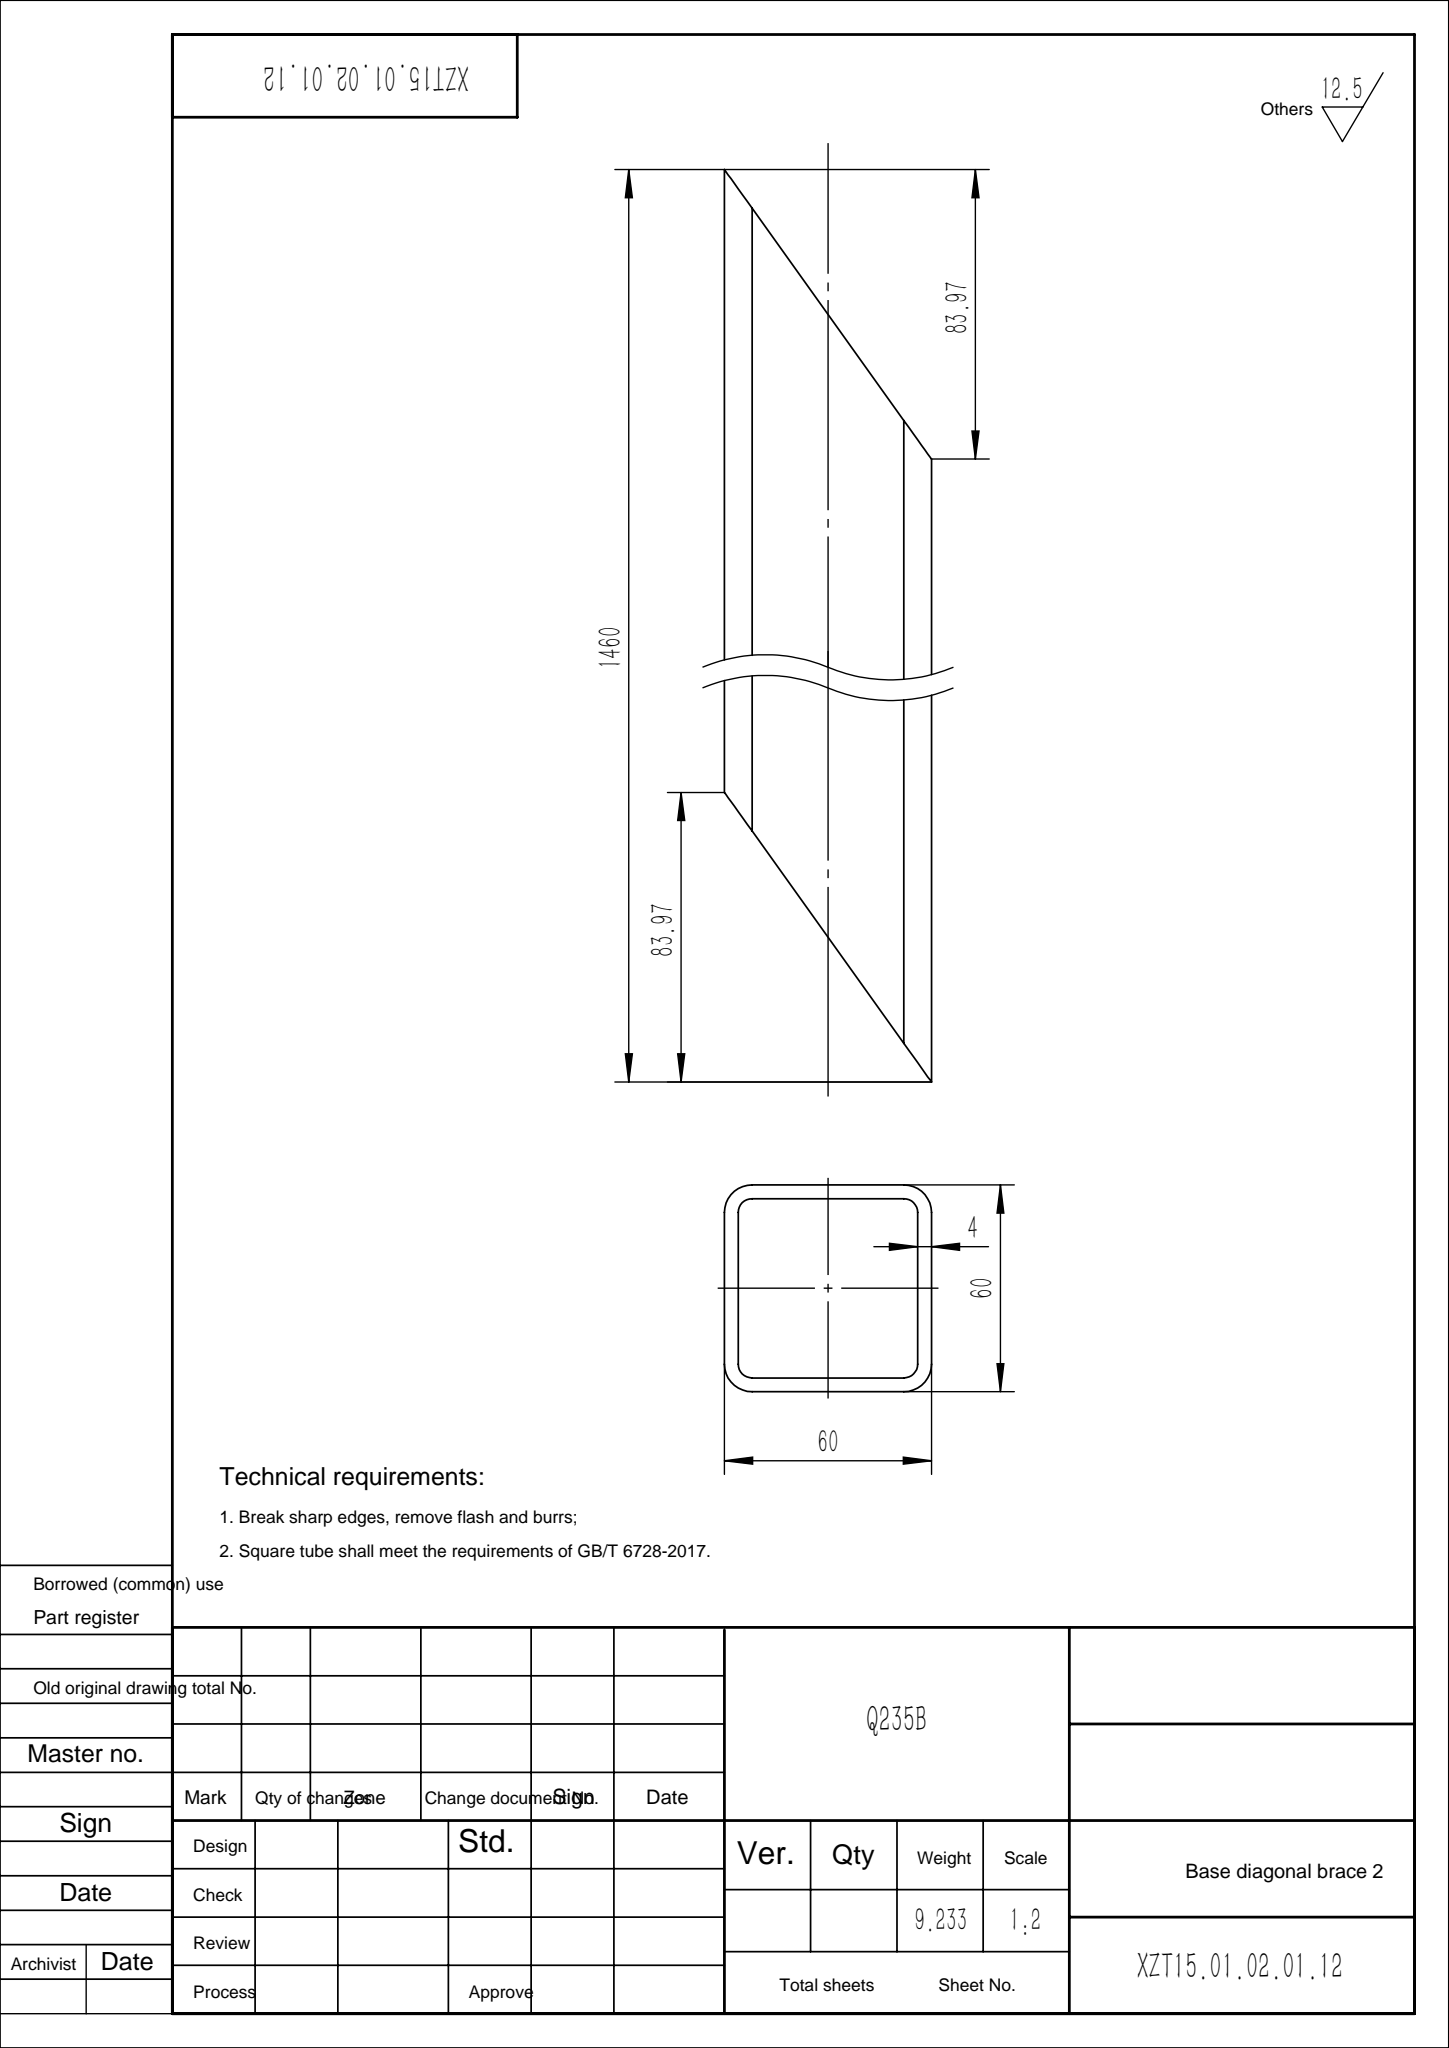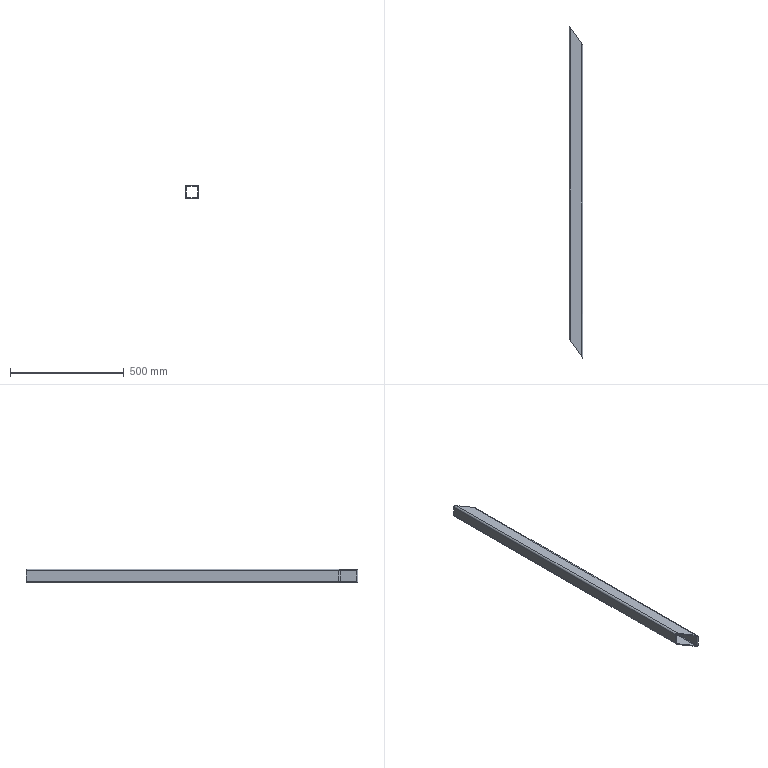Part | SolidWorks | features ICE 1, WeldMemberFeat 1, WeldmentFeature 1 | 1 solid | 18 faces | box 60 x 1460 x 60 mm | volume 1176227 mm3 | plane 10 | cylinder 8 | commonest cylinder face diameters 8 x4 16 x4
STEP:
#1=CARTESIAN_POINT('',(30.,1376.031,-22.));
#2=VERTEX_POINT('',#1);
#3=CARTESIAN_POINT('',(30.,0.,-22.));
#4=VERTEX_POINT('',#3);
#5=CARTESIAN_POINT('',(30.,1460.,-22.));
#6=DIRECTION('',(0.,-1.,0.));
#7=VECTOR('',#6,1000.);
#8=LINE('',#5,#7);
#9=EDGE_CURVE('',#2,#4,#8,.T.);
#10=ORIENTED_EDGE('',*,*,#9,.F.);
#11=CARTESIAN_POINT('',(30.,1376.031,22.));
#12=VERTEX_POINT('',#11);
#13=CARTESIAN_POINT('',(30.,1376.031,-30.));
#14=DIRECTION('',(0.,0.,1.));
#15=VECTOR('',#14,1000.);
#16=LINE('',#13,#15);
#17=EDGE_CURVE('',#2,#12,#16,.T.);
#18=ORIENTED_EDGE('',*,*,#17,.T.);
#19=CARTESIAN_POINT('',(30.,0.,22.));
#20=VERTEX_POINT('',#19);
#21=CARTESIAN_POINT('',(30.,1460.,22.));
#22=DIRECTION('',(0.,-1.,0.));
#23=VECTOR('',#22,1000.);
#24=LINE('',#21,#23);
#25=EDGE_CURVE('',#12,#20,#24,.T.);
#26=ORIENTED_EDGE('',*,*,#25,.T.);
#27=CARTESIAN_POINT('',(30.,0.,-22.));
#28=DIRECTION('',(0.,0.,-1.));
#29=VECTOR('',#28,1000.);
#30=LINE('',#27,#29);
#31=EDGE_CURVE('',#20,#4,#30,.T.);
#32=ORIENTED_EDGE('',*,*,#31,.T.);
#33=EDGE_LOOP('',(#10,#18,#26,#32));
#34=FACE_OUTER_BOUND('',#33,.T.);
#35=CARTESIAN_POINT('',(30.,1460.,-22.));
#36=DIRECTION('',(-1.,0.,0.));
#37=DIRECTION('',(0.,0.,1.));
#38=AXIS2_PLACEMENT_3D('',#35,#36,#37);
#39=PLANE('',#38);
#40=ADVANCED_FACE('',(#34),#39,.F.);
#41=CARTESIAN_POINT('',(-30.,1460.,-22.));
#42=VERTEX_POINT('',#41);
#43=CARTESIAN_POINT('',(-30.,83.969,-22.));
#44=VERTEX_POINT('',#43);
#45=CARTESIAN_POINT('',(-30.,1460.,-22.));
#46=DIRECTION('',(0.,-1.,0.));
#47=VECTOR('',#46,1000.);
#48=LINE('',#45,#47);
#49=EDGE_CURVE('',#42,#44,#48,.T.);
#50=ORIENTED_EDGE('',*,*,#49,.T.);
#51=CARTESIAN_POINT('',(-30.,83.969,22.));
#52=VERTEX_POINT('',#51);
#53=CARTESIAN_POINT('',(-30.,83.969,-30.));
#54=DIRECTION('',(0.,0.,1.));
#55=VECTOR('',#54,1000.);
#56=LINE('',#53,#55);
#57=EDGE_CURVE('',#44,#52,#56,.T.);
#58=ORIENTED_EDGE('',*,*,#57,.T.);
#59=CARTESIAN_POINT('',(-30.,1460.,22.));
#60=VERTEX_POINT('',#59);
#61=CARTESIAN_POINT('',(-30.,1460.,22.));
#62=DIRECTION('',(0.,-1.,0.));
#63=VECTOR('',#62,1000.);
#64=LINE('',#61,#63);
#65=EDGE_CURVE('',#60,#52,#64,.T.);
#66=ORIENTED_EDGE('',*,*,#65,.F.);
#67=CARTESIAN_POINT('',(-30.,1460.,22.));
#68=DIRECTION('',(0.,0.,1.));
#69=VECTOR('',#68,1000.);
#70=LINE('',#67,#69);
#71=EDGE_CURVE('',#42,#60,#70,.T.);
#72=ORIENTED_EDGE('',*,*,#71,.F.);
#73=EDGE_LOOP('',(#50,#58,#66,#72));
#74=FACE_OUTER_BOUND('',#73,.T.);
#75=CARTESIAN_POINT('',(-30.,1460.,22.));
#76=DIRECTION('',(1.,0.,0.));
#77=DIRECTION('',(0.,0.,-1.));
#78=AXIS2_PLACEMENT_3D('',#75,#76,#77);
#79=PLANE('',#78);
#80=ADVANCED_FACE('',(#74),#79,.F.);
#81=ORIENTED_EDGE('',*,*,#49,.F.);
#82=CARTESIAN_POINT('',(-22.,1448.804,-30.));
#83=VERTEX_POINT('',#82);
#84=CARTESIAN_POINT('',(-30.,1460.,-22.));
#85=CARTESIAN_POINT('',(-30.,1460.,-26.686));
#86=CARTESIAN_POINT('',(-26.686,1455.363,-30.));
#87=CARTESIAN_POINT('',(-22.,1448.804,-30.));
#88=(BOUNDED_CURVE()B_SPLINE_CURVE(3,(#84,#85,#86,#87),.UNSPECIFIED.,.F.,.F.)B_SPLINE_CURVE_WITH_KNOTS((4,4),(3.142,4.712),.UNSPECIFIED.)CURVE()GEOMETRIC_REPRESENTATION_ITEM()RATIONAL_B_SPLINE_CURVE((1.,0.8047,0.8047,1.))REPRESENTATION_ITEM(''));
#89=EDGE_CURVE('',#42,#83,#88,.T.);
#90=ORIENTED_EDGE('',*,*,#89,.T.);
#91=CARTESIAN_POINT('',(-22.,72.773,-30.));
#92=VERTEX_POINT('',#91);
#93=CARTESIAN_POINT('',(-22.,1460.,-30.));
#94=DIRECTION('',(0.,-1.,0.));
#95=VECTOR('',#94,1000.);
#96=LINE('',#93,#95);
#97=EDGE_CURVE('',#83,#92,#96,.T.);
#98=ORIENTED_EDGE('',*,*,#97,.T.);
#99=CARTESIAN_POINT('',(-22.,72.773,-30.));
#100=CARTESIAN_POINT('',(-26.686,79.331,-30.));
#101=CARTESIAN_POINT('',(-30.,83.969,-26.686));
#102=CARTESIAN_POINT('',(-30.,83.969,-22.));
#103=(BOUNDED_CURVE()B_SPLINE_CURVE(3,(#99,#100,#101,#102),.UNSPECIFIED.,.F.,.F.)B_SPLINE_CURVE_WITH_KNOTS((4,4),(1.571,3.142),.UNSPECIFIED.)CURVE()GEOMETRIC_REPRESENTATION_ITEM()RATIONAL_B_SPLINE_CURVE((1.,0.8047,0.8047,1.))REPRESENTATION_ITEM(''));
#104=EDGE_CURVE('',#92,#44,#103,.T.);
#105=ORIENTED_EDGE('',*,*,#104,.T.);
#106=EDGE_LOOP('',(#81,#90,#98,#105));
#107=FACE_OUTER_BOUND('',#106,.T.);
#108=CARTESIAN_POINT('',(-22.,1460.,-22.));
#109=DIRECTION('',(0.,-1.,0.));
#110=DIRECTION('',(0.,0.,-1.));
#111=AXIS2_PLACEMENT_3D('',#108,#109,#110);
#112=CYLINDRICAL_SURFACE('',#111,8.);
#113=ADVANCED_FACE('',(#107),#112,.T.);
#114=ORIENTED_EDGE('',*,*,#97,.F.);
#115=CARTESIAN_POINT('',(22.,1387.227,-30.));
#116=VERTEX_POINT('',#115);
#117=CARTESIAN_POINT('',(-30.,1460.,-30.));
#118=DIRECTION('',(0.5814,-0.8136,0.));
#119=VECTOR('',#118,1000.);
#120=LINE('',#117,#119);
#121=EDGE_CURVE('',#83,#116,#120,.T.);
#122=ORIENTED_EDGE('',*,*,#121,.T.);
#123=CARTESIAN_POINT('',(22.,11.196,-30.));
#124=VERTEX_POINT('',#123);
#125=CARTESIAN_POINT('',(22.,1460.,-30.));
#126=DIRECTION('',(0.,-1.,0.));
#127=VECTOR('',#126,1000.);
#128=LINE('',#125,#127);
#129=EDGE_CURVE('',#116,#124,#128,.T.);
#130=ORIENTED_EDGE('',*,*,#129,.T.);
#131=CARTESIAN_POINT('',(-30.,83.969,-30.));
#132=DIRECTION('',(-0.5814,0.8136,0.));
#133=VECTOR('',#132,1000.);
#134=LINE('',#131,#133);
#135=EDGE_CURVE('',#124,#92,#134,.T.);
#136=ORIENTED_EDGE('',*,*,#135,.T.);
#137=EDGE_LOOP('',(#114,#122,#130,#136));
#138=FACE_OUTER_BOUND('',#137,.T.);
#139=CARTESIAN_POINT('',(22.,1460.,-30.));
#140=DIRECTION('',(0.,0.,1.));
#141=DIRECTION('',(1.,0.,0.));
#142=AXIS2_PLACEMENT_3D('',#139,#140,#141);
#143=PLANE('',#142);
#144=ADVANCED_FACE('',(#138),#143,.F.);
#145=ORIENTED_EDGE('',*,*,#129,.F.);
#146=CARTESIAN_POINT('',(22.,1387.227,-30.));
#147=CARTESIAN_POINT('',(26.686,1380.669,-30.));
#148=CARTESIAN_POINT('',(30.,1376.031,-26.686));
#149=CARTESIAN_POINT('',(30.,1376.031,-22.));
#150=(BOUNDED_CURVE()B_SPLINE_CURVE(3,(#146,#147,#148,#149),.UNSPECIFIED.,.F.,.F.)B_SPLINE_CURVE_WITH_KNOTS((4,4),(4.712,6.283),.UNSPECIFIED.)CURVE()GEOMETRIC_REPRESENTATION_ITEM()RATIONAL_B_SPLINE_CURVE((1.,0.8047,0.8047,1.))REPRESENTATION_ITEM(''));
#151=EDGE_CURVE('',#116,#2,#150,.T.);
#152=ORIENTED_EDGE('',*,*,#151,.T.);
#153=ORIENTED_EDGE('',*,*,#9,.T.);
#154=CARTESIAN_POINT('',(30.,0.,-22.));
#155=CARTESIAN_POINT('',(30.,0.,-26.686));
#156=CARTESIAN_POINT('',(26.686,4.637,-30.));
#157=CARTESIAN_POINT('',(22.,11.196,-30.));
#158=(BOUNDED_CURVE()B_SPLINE_CURVE(3,(#154,#155,#156,#157),.UNSPECIFIED.,.F.,.T.)B_SPLINE_CURVE_WITH_KNOTS((4,4),(0.,1.571),.UNSPECIFIED.)CURVE()GEOMETRIC_REPRESENTATION_ITEM()RATIONAL_B_SPLINE_CURVE((1.,0.8047,0.8047,1.))REPRESENTATION_ITEM(''));
#159=EDGE_CURVE('',#4,#124,#158,.T.);
#160=ORIENTED_EDGE('',*,*,#159,.T.);
#161=EDGE_LOOP('',(#145,#152,#153,#160));
#162=FACE_OUTER_BOUND('',#161,.T.);
#163=CARTESIAN_POINT('',(22.,1460.,-22.));
#164=DIRECTION('',(0.,-1.,0.));
#165=DIRECTION('',(0.,0.,-1.));
#166=AXIS2_PLACEMENT_3D('',#163,#164,#165);
#167=CYLINDRICAL_SURFACE('',#166,8.);
#168=ADVANCED_FACE('',(#162),#167,.T.);
#169=ORIENTED_EDGE('',*,*,#25,.F.);
#170=CARTESIAN_POINT('',(22.,1387.227,30.));
#171=VERTEX_POINT('',#170);
#172=CARTESIAN_POINT('',(30.,1376.031,22.));
#173=CARTESIAN_POINT('',(30.,1376.031,26.686));
#174=CARTESIAN_POINT('',(26.686,1380.669,30.));
#175=CARTESIAN_POINT('',(22.,1387.227,30.));
#176=(BOUNDED_CURVE()B_SPLINE_CURVE(3,(#172,#173,#174,#175),.UNSPECIFIED.,.F.,.F.)B_SPLINE_CURVE_WITH_KNOTS((4,4),(0.,1.571),.UNSPECIFIED.)CURVE()GEOMETRIC_REPRESENTATION_ITEM()RATIONAL_B_SPLINE_CURVE((1.,0.8047,0.8047,1.))REPRESENTATION_ITEM(''));
#177=EDGE_CURVE('',#12,#171,#176,.T.);
#178=ORIENTED_EDGE('',*,*,#177,.T.);
#179=CARTESIAN_POINT('',(22.,11.196,30.));
#180=VERTEX_POINT('',#179);
#181=CARTESIAN_POINT('',(22.,1460.,30.));
#182=DIRECTION('',(0.,-1.,0.));
#183=VECTOR('',#182,1000.);
#184=LINE('',#181,#183);
#185=EDGE_CURVE('',#171,#180,#184,.T.);
#186=ORIENTED_EDGE('',*,*,#185,.T.);
#187=CARTESIAN_POINT('',(22.,11.196,30.));
#188=CARTESIAN_POINT('',(26.686,4.637,30.));
#189=CARTESIAN_POINT('',(30.,0.,26.686));
#190=CARTESIAN_POINT('',(30.,0.,22.));
#191=(BOUNDED_CURVE()B_SPLINE_CURVE(3,(#187,#188,#189,#190),.UNSPECIFIED.,.F.,.T.)B_SPLINE_CURVE_WITH_KNOTS((4,4),(4.712,6.283),.UNSPECIFIED.)CURVE()GEOMETRIC_REPRESENTATION_ITEM()RATIONAL_B_SPLINE_CURVE((1.,0.8047,0.8047,1.))REPRESENTATION_ITEM(''));
#192=EDGE_CURVE('',#180,#20,#191,.T.);
#193=ORIENTED_EDGE('',*,*,#192,.T.);
#194=EDGE_LOOP('',(#169,#178,#186,#193));
#195=FACE_OUTER_BOUND('',#194,.T.);
#196=CARTESIAN_POINT('',(22.,1460.,22.));
#197=DIRECTION('',(0.,-1.,0.));
#198=DIRECTION('',(0.,0.,-1.));
#199=AXIS2_PLACEMENT_3D('',#196,#197,#198);
#200=CYLINDRICAL_SURFACE('',#199,8.);
#201=ADVANCED_FACE('',(#195),#200,.T.);
#202=ORIENTED_EDGE('',*,*,#185,.F.);
#203=CARTESIAN_POINT('',(-22.,1448.804,30.));
#204=VERTEX_POINT('',#203);
#205=CARTESIAN_POINT('',(-27.296,1456.216,30.));
#206=DIRECTION('',(-0.5814,0.8136,0.));
#207=VECTOR('',#206,1000.);
#208=LINE('',#205,#207);
#209=EDGE_CURVE('',#171,#204,#208,.T.);
#210=ORIENTED_EDGE('',*,*,#209,.T.);
#211=CARTESIAN_POINT('',(-22.,72.773,30.));
#212=VERTEX_POINT('',#211);
#213=CARTESIAN_POINT('',(-22.,1460.,30.));
#214=DIRECTION('',(0.,-1.,0.));
#215=VECTOR('',#214,1000.);
#216=LINE('',#213,#215);
#217=EDGE_CURVE('',#204,#212,#216,.T.);
#218=ORIENTED_EDGE('',*,*,#217,.T.);
#219=CARTESIAN_POINT('',(-678.2,991.11,30.));
#220=DIRECTION('',(0.5814,-0.8136,0.));
#221=VECTOR('',#220,1000.);
#222=LINE('',#219,#221);
#223=EDGE_CURVE('',#212,#180,#222,.T.);
#224=ORIENTED_EDGE('',*,*,#223,.T.);
#225=EDGE_LOOP('',(#202,#210,#218,#224));
#226=FACE_OUTER_BOUND('',#225,.T.);
#227=CARTESIAN_POINT('',(-22.,1460.,30.));
#228=DIRECTION('',(0.,0.,-1.));
#229=DIRECTION('',(-1.,0.,0.));
#230=AXIS2_PLACEMENT_3D('',#227,#228,#229);
#231=PLANE('',#230);
#232=ADVANCED_FACE('',(#226),#231,.F.);
#233=ORIENTED_EDGE('',*,*,#217,.F.);
#234=CARTESIAN_POINT('',(-22.,1448.804,30.));
#235=CARTESIAN_POINT('',(-26.686,1455.363,30.));
#236=CARTESIAN_POINT('',(-30.,1460.,26.686));
#237=CARTESIAN_POINT('',(-30.,1460.,22.));
#238=(BOUNDED_CURVE()B_SPLINE_CURVE(3,(#234,#235,#236,#237),.UNSPECIFIED.,.F.,.T.)B_SPLINE_CURVE_WITH_KNOTS((4,4),(1.571,3.142),.UNSPECIFIED.)CURVE()GEOMETRIC_REPRESENTATION_ITEM()RATIONAL_B_SPLINE_CURVE((1.,0.8047,0.8047,1.))REPRESENTATION_ITEM(''));
#239=EDGE_CURVE('',#204,#60,#238,.T.);
#240=ORIENTED_EDGE('',*,*,#239,.T.);
#241=ORIENTED_EDGE('',*,*,#65,.T.);
#242=CARTESIAN_POINT('',(-30.,83.969,22.));
#243=CARTESIAN_POINT('',(-30.,83.969,26.686));
#244=CARTESIAN_POINT('',(-26.686,79.331,30.));
#245=CARTESIAN_POINT('',(-22.,72.773,30.));
#246=(BOUNDED_CURVE()B_SPLINE_CURVE(3,(#242,#243,#244,#245),.UNSPECIFIED.,.F.,.T.)B_SPLINE_CURVE_WITH_KNOTS((4,4),(3.142,4.712),.UNSPECIFIED.)CURVE()GEOMETRIC_REPRESENTATION_ITEM()RATIONAL_B_SPLINE_CURVE((1.,0.8047,0.8047,1.))REPRESENTATION_ITEM(''));
#247=EDGE_CURVE('',#52,#212,#246,.T.);
#248=ORIENTED_EDGE('',*,*,#247,.T.);
#249=EDGE_LOOP('',(#233,#240,#241,#248));
#250=FACE_OUTER_BOUND('',#249,.T.);
#251=CARTESIAN_POINT('',(-22.,1460.,22.));
#252=DIRECTION('',(0.,-1.,0.));
#253=DIRECTION('',(0.,0.,-1.));
#254=AXIS2_PLACEMENT_3D('',#251,#252,#253);
#255=CYLINDRICAL_SURFACE('',#254,8.);
#256=ADVANCED_FACE('',(#250),#255,.T.);
#257=CARTESIAN_POINT('',(22.,11.196,26.));
#258=VERTEX_POINT('',#257);
#259=CARTESIAN_POINT('',(26.,5.598,22.));
#260=VERTEX_POINT('',#259);
#261=CARTESIAN_POINT('',(22.,11.196,26.));
#262=CARTESIAN_POINT('',(24.343,7.917,26.));
#263=CARTESIAN_POINT('',(26.,5.598,24.343));
#264=CARTESIAN_POINT('',(26.,5.598,22.));
#265=(BOUNDED_CURVE()B_SPLINE_CURVE(3,(#261,#262,#263,#264),.UNSPECIFIED.,.F.,.T.)B_SPLINE_CURVE_WITH_KNOTS((4,4),(4.712,6.283),.UNSPECIFIED.)CURVE()GEOMETRIC_REPRESENTATION_ITEM()RATIONAL_B_SPLINE_CURVE((1.,0.8047,0.8047,1.))REPRESENTATION_ITEM(''));
#266=EDGE_CURVE('',#258,#260,#265,.T.);
#267=ORIENTED_EDGE('',*,*,#266,.T.);
#268=CARTESIAN_POINT('',(26.,5.598,-22.));
#269=VERTEX_POINT('',#268);
#270=CARTESIAN_POINT('',(26.,5.598,-22.));
#271=DIRECTION('',(0.,0.,-1.));
#272=VECTOR('',#271,1000.);
#273=LINE('',#270,#272);
#274=EDGE_CURVE('',#260,#269,#273,.T.);
#275=ORIENTED_EDGE('',*,*,#274,.T.);
#276=CARTESIAN_POINT('',(22.,11.196,-26.));
#277=VERTEX_POINT('',#276);
#278=CARTESIAN_POINT('',(26.,5.598,-22.));
#279=CARTESIAN_POINT('',(26.,5.598,-24.343));
#280=CARTESIAN_POINT('',(24.343,7.917,-26.));
#281=CARTESIAN_POINT('',(22.,11.196,-26.));
#282=(BOUNDED_CURVE()B_SPLINE_CURVE(3,(#278,#279,#280,#281),.UNSPECIFIED.,.F.,.T.)B_SPLINE_CURVE_WITH_KNOTS((4,4),(0.,1.571),.UNSPECIFIED.)CURVE()GEOMETRIC_REPRESENTATION_ITEM()RATIONAL_B_SPLINE_CURVE((1.,0.8047,0.8047,1.))REPRESENTATION_ITEM(''));
#283=EDGE_CURVE('',#269,#277,#282,.T.);
#284=ORIENTED_EDGE('',*,*,#283,.T.);
#285=CARTESIAN_POINT('',(-22.,72.773,-26.));
#286=VERTEX_POINT('',#285);
#287=CARTESIAN_POINT('',(-663.328,970.297,-26.));
#288=DIRECTION('',(-0.5814,0.8136,0.));
#289=VECTOR('',#288,1000.);
#290=LINE('',#287,#289);
#291=EDGE_CURVE('',#277,#286,#290,.T.);
#292=ORIENTED_EDGE('',*,*,#291,.T.);
#293=CARTESIAN_POINT('',(-26.,78.371,-22.));
#294=VERTEX_POINT('',#293);
#295=CARTESIAN_POINT('',(-22.,72.773,-26.));
#296=CARTESIAN_POINT('',(-24.343,76.052,-26.));
#297=CARTESIAN_POINT('',(-26.,78.371,-24.343));
#298=CARTESIAN_POINT('',(-26.,78.371,-22.));
#299=(BOUNDED_CURVE()B_SPLINE_CURVE(3,(#295,#296,#297,#298),.UNSPECIFIED.,.F.,.F.)B_SPLINE_CURVE_WITH_KNOTS((4,4),(1.571,3.142),.UNSPECIFIED.)CURVE()GEOMETRIC_REPRESENTATION_ITEM()RATIONAL_B_SPLINE_CURVE((1.,0.8047,0.8047,1.))REPRESENTATION_ITEM(''));
#300=EDGE_CURVE('',#286,#294,#299,.T.);
#301=ORIENTED_EDGE('',*,*,#300,.T.);
#302=CARTESIAN_POINT('',(-26.,78.371,22.));
#303=VERTEX_POINT('',#302);
#304=CARTESIAN_POINT('',(-26.,78.371,22.));
#305=DIRECTION('',(0.,0.,1.));
#306=VECTOR('',#305,1000.);
#307=LINE('',#304,#306);
#308=EDGE_CURVE('',#294,#303,#307,.T.);
#309=ORIENTED_EDGE('',*,*,#308,.T.);
#310=CARTESIAN_POINT('',(-22.,72.773,26.));
#311=VERTEX_POINT('',#310);
#312=CARTESIAN_POINT('',(-26.,78.371,22.));
#313=CARTESIAN_POINT('',(-26.,78.371,24.343));
#314=CARTESIAN_POINT('',(-24.343,76.052,26.));
#315=CARTESIAN_POINT('',(-22.,72.773,26.));
#316=(BOUNDED_CURVE()B_SPLINE_CURVE(3,(#312,#313,#314,#315),.UNSPECIFIED.,.F.,.T.)B_SPLINE_CURVE_WITH_KNOTS((4,4),(3.142,4.712),.UNSPECIFIED.)CURVE()GEOMETRIC_REPRESENTATION_ITEM()RATIONAL_B_SPLINE_CURVE((1.,0.8047,0.8047,1.))REPRESENTATION_ITEM(''));
#317=EDGE_CURVE('',#303,#311,#316,.T.);
#318=ORIENTED_EDGE('',*,*,#317,.T.);
#319=CARTESIAN_POINT('',(-678.2,991.11,26.));
#320=DIRECTION('',(0.5814,-0.8136,0.));
#321=VECTOR('',#320,1000.);
#322=LINE('',#319,#321);
#323=EDGE_CURVE('',#311,#258,#322,.T.);
#324=ORIENTED_EDGE('',*,*,#323,.T.);
#325=EDGE_LOOP('',(#267,#275,#284,#292,#301,#309,#318,#324));
#326=FACE_BOUND('',#325,.T.);
#327=ORIENTED_EDGE('',*,*,#57,.F.);
#328=ORIENTED_EDGE('',*,*,#104,.F.);
#329=ORIENTED_EDGE('',*,*,#135,.F.);
#330=ORIENTED_EDGE('',*,*,#159,.F.);
#331=ORIENTED_EDGE('',*,*,#31,.F.);
#332=ORIENTED_EDGE('',*,*,#192,.F.);
#333=ORIENTED_EDGE('',*,*,#223,.F.);
#334=ORIENTED_EDGE('',*,*,#247,.F.);
#335=EDGE_LOOP('',(#327,#328,#329,#330,#331,#332,#333,#334));
#336=FACE_OUTER_BOUND('',#335,.T.);
#337=CARTESIAN_POINT('',(-30.,83.969,-30.));
#338=DIRECTION('',(0.8136,0.5814,0.));
#339=DIRECTION('',(-0.5814,0.8136,0.));
#340=AXIS2_PLACEMENT_3D('',#337,#338,#339);
#341=PLANE('',#340);
#342=ADVANCED_FACE('',(#326,#336),#341,.F.);
#343=CARTESIAN_POINT('',(26.,1381.629,22.));
#344=VERTEX_POINT('',#343);
#345=CARTESIAN_POINT('',(22.,1387.227,26.));
#346=VERTEX_POINT('',#345);
#347=CARTESIAN_POINT('',(26.,1381.629,22.));
#348=CARTESIAN_POINT('',(26.,1381.629,24.343));
#349=CARTESIAN_POINT('',(24.343,1383.948,26.));
#350=CARTESIAN_POINT('',(22.,1387.227,26.));
#351=(BOUNDED_CURVE()B_SPLINE_CURVE(3,(#347,#348,#349,#350),.UNSPECIFIED.,.F.,.T.)B_SPLINE_CURVE_WITH_KNOTS((4,4),(0.,1.571),.UNSPECIFIED.)CURVE()GEOMETRIC_REPRESENTATION_ITEM()RATIONAL_B_SPLINE_CURVE((1.,0.8047,0.8047,1.))REPRESENTATION_ITEM(''));
#352=EDGE_CURVE('',#344,#346,#351,.T.);
#353=ORIENTED_EDGE('',*,*,#352,.T.);
#354=CARTESIAN_POINT('',(-22.,1448.804,26.));
#355=VERTEX_POINT('',#354);
#356=CARTESIAN_POINT('',(-27.296,1456.216,26.));
#357=DIRECTION('',(-0.5814,0.8136,0.));
#358=VECTOR('',#357,1000.);
#359=LINE('',#356,#358);
#360=EDGE_CURVE('',#346,#355,#359,.T.);
#361=ORIENTED_EDGE('',*,*,#360,.T.);
#362=CARTESIAN_POINT('',(-26.,1454.402,22.));
#363=VERTEX_POINT('',#362);
#364=CARTESIAN_POINT('',(-22.,1448.804,26.));
#365=CARTESIAN_POINT('',(-24.343,1452.083,26.));
#366=CARTESIAN_POINT('',(-26.,1454.402,24.343));
#367=CARTESIAN_POINT('',(-26.,1454.402,22.));
#368=(BOUNDED_CURVE()B_SPLINE_CURVE(3,(#364,#365,#366,#367),.UNSPECIFIED.,.F.,.F.)B_SPLINE_CURVE_WITH_KNOTS((4,4),(1.571,3.142),.UNSPECIFIED.)CURVE()GEOMETRIC_REPRESENTATION_ITEM()RATIONAL_B_SPLINE_CURVE((1.,0.8047,0.8047,1.))REPRESENTATION_ITEM(''));
#369=EDGE_CURVE('',#355,#363,#368,.T.);
#370=ORIENTED_EDGE('',*,*,#369,.T.);
#371=CARTESIAN_POINT('',(-26.,1454.402,-22.));
#372=VERTEX_POINT('',#371);
#373=CARTESIAN_POINT('',(-26.,1454.402,22.));
#374=DIRECTION('',(0.,0.,-1.));
#375=VECTOR('',#374,1000.);
#376=LINE('',#373,#375);
#377=EDGE_CURVE('',#363,#372,#376,.T.);
#378=ORIENTED_EDGE('',*,*,#377,.T.);
#379=CARTESIAN_POINT('',(-22.,1448.804,-26.));
#380=VERTEX_POINT('',#379);
#381=CARTESIAN_POINT('',(-26.,1454.402,-22.));
#382=CARTESIAN_POINT('',(-26.,1454.402,-24.343));
#383=CARTESIAN_POINT('',(-24.343,1452.083,-26.));
#384=CARTESIAN_POINT('',(-22.,1448.804,-26.));
#385=(BOUNDED_CURVE()B_SPLINE_CURVE(3,(#381,#382,#383,#384),.UNSPECIFIED.,.F.,.F.)B_SPLINE_CURVE_WITH_KNOTS((4,4),(3.142,4.712),.UNSPECIFIED.)CURVE()GEOMETRIC_REPRESENTATION_ITEM()RATIONAL_B_SPLINE_CURVE((1.,0.8047,0.8047,1.))REPRESENTATION_ITEM(''));
#386=EDGE_CURVE('',#372,#380,#385,.T.);
#387=ORIENTED_EDGE('',*,*,#386,.T.);
#388=CARTESIAN_POINT('',(22.,1387.227,-26.));
#389=VERTEX_POINT('',#388);
#390=CARTESIAN_POINT('',(-12.424,1435.402,-26.));
#391=DIRECTION('',(0.5814,-0.8136,0.));
#392=VECTOR('',#391,1000.);
#393=LINE('',#390,#392);
#394=EDGE_CURVE('',#380,#389,#393,.T.);
#395=ORIENTED_EDGE('',*,*,#394,.T.);
#396=CARTESIAN_POINT('',(26.,1381.629,-22.));
#397=VERTEX_POINT('',#396);
#398=CARTESIAN_POINT('',(22.,1387.227,-26.));
#399=CARTESIAN_POINT('',(24.343,1383.948,-26.));
#400=CARTESIAN_POINT('',(26.,1381.629,-24.343));
#401=CARTESIAN_POINT('',(26.,1381.629,-22.));
#402=(BOUNDED_CURVE()B_SPLINE_CURVE(3,(#398,#399,#400,#401),.UNSPECIFIED.,.F.,.F.)B_SPLINE_CURVE_WITH_KNOTS((4,4),(4.712,6.283),.UNSPECIFIED.)CURVE()GEOMETRIC_REPRESENTATION_ITEM()RATIONAL_B_SPLINE_CURVE((1.,0.8047,0.8047,1.))REPRESENTATION_ITEM(''));
#403=EDGE_CURVE('',#389,#397,#402,.T.);
#404=ORIENTED_EDGE('',*,*,#403,.T.);
#405=CARTESIAN_POINT('',(26.,1381.629,-22.));
#406=DIRECTION('',(0.,0.,1.));
#407=VECTOR('',#406,1000.);
#408=LINE('',#405,#407);
#409=EDGE_CURVE('',#397,#344,#408,.T.);
#410=ORIENTED_EDGE('',*,*,#409,.T.);
#411=EDGE_LOOP('',(#353,#361,#370,#378,#387,#395,#404,#410));
#412=FACE_BOUND('',#411,.T.);
#413=ORIENTED_EDGE('',*,*,#209,.F.);
#414=ORIENTED_EDGE('',*,*,#177,.F.);
#415=ORIENTED_EDGE('',*,*,#17,.F.);
#416=ORIENTED_EDGE('',*,*,#151,.F.);
#417=ORIENTED_EDGE('',*,*,#121,.F.);
#418=ORIENTED_EDGE('',*,*,#89,.F.);
#419=ORIENTED_EDGE('',*,*,#71,.T.);
#420=ORIENTED_EDGE('',*,*,#239,.F.);
#421=EDGE_LOOP('',(#413,#414,#415,#416,#417,#418,#419,#420));
#422=FACE_OUTER_BOUND('',#421,.T.);
#423=CARTESIAN_POINT('',(-30.,1460.,-30.));
#424=DIRECTION('',(-0.8136,-0.5814,0.));
#425=DIRECTION('',(0.5814,-0.8136,0.));
#426=AXIS2_PLACEMENT_3D('',#423,#424,#425);
#427=PLANE('',#426);
#428=ADVANCED_FACE('',(#412,#422),#427,.F.);
#429=ORIENTED_EDGE('',*,*,#352,.F.);
#430=CARTESIAN_POINT('',(26.,1460.,22.));
#431=DIRECTION('',(0.,-1.,0.));
#432=VECTOR('',#431,1000.);
#433=LINE('',#430,#432);
#434=EDGE_CURVE('',#344,#260,#433,.T.);
#435=ORIENTED_EDGE('',*,*,#434,.T.);
#436=ORIENTED_EDGE('',*,*,#266,.F.);
#437=CARTESIAN_POINT('',(22.,1460.,26.));
#438=DIRECTION('',(0.,-1.,0.));
#439=VECTOR('',#438,1000.);
#440=LINE('',#437,#439);
#441=EDGE_CURVE('',#346,#258,#440,.T.);
#442=ORIENTED_EDGE('',*,*,#441,.F.);
#443=EDGE_LOOP('',(#429,#435,#436,#442));
#444=FACE_OUTER_BOUND('',#443,.T.);
#445=CARTESIAN_POINT('',(22.,1460.,22.));
#446=DIRECTION('',(0.,-1.,0.));
#447=DIRECTION('',(0.,0.,-1.));
#448=AXIS2_PLACEMENT_3D('',#445,#446,#447);
#449=CYLINDRICAL_SURFACE('',#448,4.);
#450=ADVANCED_FACE('',(#444),#449,.F.);
#451=ORIENTED_EDGE('',*,*,#360,.F.);
#452=ORIENTED_EDGE('',*,*,#441,.T.);
#453=ORIENTED_EDGE('',*,*,#323,.F.);
#454=CARTESIAN_POINT('',(-22.,1460.,26.));
#455=DIRECTION('',(0.,-1.,0.));
#456=VECTOR('',#455,1000.);
#457=LINE('',#454,#456);
#458=EDGE_CURVE('',#355,#311,#457,.T.);
#459=ORIENTED_EDGE('',*,*,#458,.F.);
#460=EDGE_LOOP('',(#451,#452,#453,#459));
#461=FACE_OUTER_BOUND('',#460,.T.);
#462=CARTESIAN_POINT('',(-22.,1460.,26.));
#463=DIRECTION('',(0.,0.,-1.));
#464=DIRECTION('',(-1.,0.,0.));
#465=AXIS2_PLACEMENT_3D('',#462,#463,#464);
#466=PLANE('',#465);
#467=ADVANCED_FACE('',(#461),#466,.T.);
#468=ORIENTED_EDGE('',*,*,#369,.F.);
#469=ORIENTED_EDGE('',*,*,#458,.T.);
#470=ORIENTED_EDGE('',*,*,#317,.F.);
#471=CARTESIAN_POINT('',(-26.,1460.,22.));
#472=DIRECTION('',(0.,-1.,0.));
#473=VECTOR('',#472,1000.);
#474=LINE('',#471,#473);
#475=EDGE_CURVE('',#363,#303,#474,.T.);
#476=ORIENTED_EDGE('',*,*,#475,.F.);
#477=EDGE_LOOP('',(#468,#469,#470,#476));
#478=FACE_OUTER_BOUND('',#477,.T.);
#479=CARTESIAN_POINT('',(-22.,1460.,22.));
#480=DIRECTION('',(0.,-1.,0.));
#481=DIRECTION('',(0.,0.,-1.));
#482=AXIS2_PLACEMENT_3D('',#479,#480,#481);
#483=CYLINDRICAL_SURFACE('',#482,4.);
#484=ADVANCED_FACE('',(#478),#483,.F.);
#485=ORIENTED_EDGE('',*,*,#377,.F.);
#486=ORIENTED_EDGE('',*,*,#475,.T.);
#487=ORIENTED_EDGE('',*,*,#308,.F.);
#488=CARTESIAN_POINT('',(-26.,1460.,-22.));
#489=DIRECTION('',(0.,-1.,0.));
#490=VECTOR('',#489,1000.);
#491=LINE('',#488,#490);
#492=EDGE_CURVE('',#372,#294,#491,.T.);
#493=ORIENTED_EDGE('',*,*,#492,.F.);
#494=EDGE_LOOP('',(#485,#486,#487,#493));
#495=FACE_OUTER_BOUND('',#494,.T.);
#496=CARTESIAN_POINT('',(-26.,1460.,22.));
#497=DIRECTION('',(1.,0.,0.));
#498=DIRECTION('',(0.,0.,-1.));
#499=AXIS2_PLACEMENT_3D('',#496,#497,#498);
#500=PLANE('',#499);
#501=ADVANCED_FACE('',(#495),#500,.T.);
#502=ORIENTED_EDGE('',*,*,#386,.F.);
#503=ORIENTED_EDGE('',*,*,#492,.T.);
#504=ORIENTED_EDGE('',*,*,#300,.F.);
#505=CARTESIAN_POINT('',(-22.,1460.,-26.));
#506=DIRECTION('',(0.,-1.,0.));
#507=VECTOR('',#506,1000.);
#508=LINE('',#505,#507);
#509=EDGE_CURVE('',#380,#286,#508,.T.);
#510=ORIENTED_EDGE('',*,*,#509,.F.);
#511=EDGE_LOOP('',(#502,#503,#504,#510));
#512=FACE_OUTER_BOUND('',#511,.T.);
#513=CARTESIAN_POINT('',(-22.,1460.,-22.));
#514=DIRECTION('',(0.,-1.,0.));
#515=DIRECTION('',(0.,0.,-1.));
#516=AXIS2_PLACEMENT_3D('',#513,#514,#515);
#517=CYLINDRICAL_SURFACE('',#516,4.);
#518=ADVANCED_FACE('',(#512),#517,.F.);
#519=ORIENTED_EDGE('',*,*,#394,.F.);
#520=ORIENTED_EDGE('',*,*,#509,.T.);
#521=ORIENTED_EDGE('',*,*,#291,.F.);
#522=CARTESIAN_POINT('',(22.,1460.,-26.));
#523=DIRECTION('',(0.,-1.,0.));
#524=VECTOR('',#523,1000.);
#525=LINE('',#522,#524);
#526=EDGE_CURVE('',#389,#277,#525,.T.);
#527=ORIENTED_EDGE('',*,*,#526,.F.);
#528=EDGE_LOOP('',(#519,#520,#521,#527));
#529=FACE_OUTER_BOUND('',#528,.T.);
#530=CARTESIAN_POINT('',(22.,1460.,-26.));
#531=DIRECTION('',(0.,0.,1.));
#532=DIRECTION('',(1.,0.,0.));
#533=AXIS2_PLACEMENT_3D('',#530,#531,#532);
#534=PLANE('',#533);
#535=ADVANCED_FACE('',(#529),#534,.T.);
#536=ORIENTED_EDGE('',*,*,#403,.F.);
#537=ORIENTED_EDGE('',*,*,#526,.T.);
#538=ORIENTED_EDGE('',*,*,#283,.F.);
#539=CARTESIAN_POINT('',(26.,1460.,-22.));
#540=DIRECTION('',(0.,-1.,0.));
#541=VECTOR('',#540,1000.);
#542=LINE('',#539,#541);
#543=EDGE_CURVE('',#397,#269,#542,.T.);
#544=ORIENTED_EDGE('',*,*,#543,.F.);
#545=EDGE_LOOP('',(#536,#537,#538,#544));
#546=FACE_OUTER_BOUND('',#545,.T.);
#547=CARTESIAN_POINT('',(22.,1460.,-22.));
#548=DIRECTION('',(0.,-1.,0.));
#549=DIRECTION('',(0.,0.,-1.));
#550=AXIS2_PLACEMENT_3D('',#547,#548,#549);
#551=CYLINDRICAL_SURFACE('',#550,4.);
#552=ADVANCED_FACE('',(#546),#551,.F.);
#553=ORIENTED_EDGE('',*,*,#409,.F.);
#554=ORIENTED_EDGE('',*,*,#543,.T.);
#555=ORIENTED_EDGE('',*,*,#274,.F.);
#556=ORIENTED_EDGE('',*,*,#434,.F.);
#557=EDGE_LOOP('',(#553,#554,#555,#556));
#558=FACE_OUTER_BOUND('',#557,.T.);
#559=CARTESIAN_POINT('',(26.,1460.,-22.));
#560=DIRECTION('',(-1.,0.,0.));
#561=DIRECTION('',(0.,0.,1.));
#562=AXIS2_PLACEMENT_3D('',#559,#560,#561);
#563=PLANE('',#562);
#564=ADVANCED_FACE('',(#558),#563,.T.);
#565=CLOSED_SHELL('',(#40,#80,#113,#144,#168,#201,#232,#256,#342,#428,#450,#467,#484,#501,#518,#535,#552,#564));
#566=MANIFOLD_SOLID_BREP('',#565);
#567=CARTESIAN_POINT('',(0.,0.,0.));
#568=DIRECTION('',(0.,0.,1.));
#569=DIRECTION('',(1.,0.,0.));
#570=AXIS2_PLACEMENT_3D('',#567,#568,#569);
#571=(LENGTH_UNIT()NAMED_UNIT(*)SI_UNIT(.MILLI.,.METRE.));
#572=UNCERTAINTY_MEASURE_WITH_UNIT(LENGTH_MEASURE(0.00001),#571,'','');
#573=(NAMED_UNIT(*)PLANE_ANGLE_UNIT()SI_UNIT($,.RADIAN.));
#574=(NAMED_UNIT(*)SI_UNIT($,.STERADIAN.)SOLID_ANGLE_UNIT());
#575=(GEOMETRIC_REPRESENTATION_CONTEXT(3)GLOBAL_UNCERTAINTY_ASSIGNED_CONTEXT((#572))GLOBAL_UNIT_ASSIGNED_CONTEXT((#571,#573,#574))REPRESENTATION_CONTEXT('',''));
#576=ADVANCED_BREP_SHAPE_REPRESENTATION('',(#566,#570),#575);